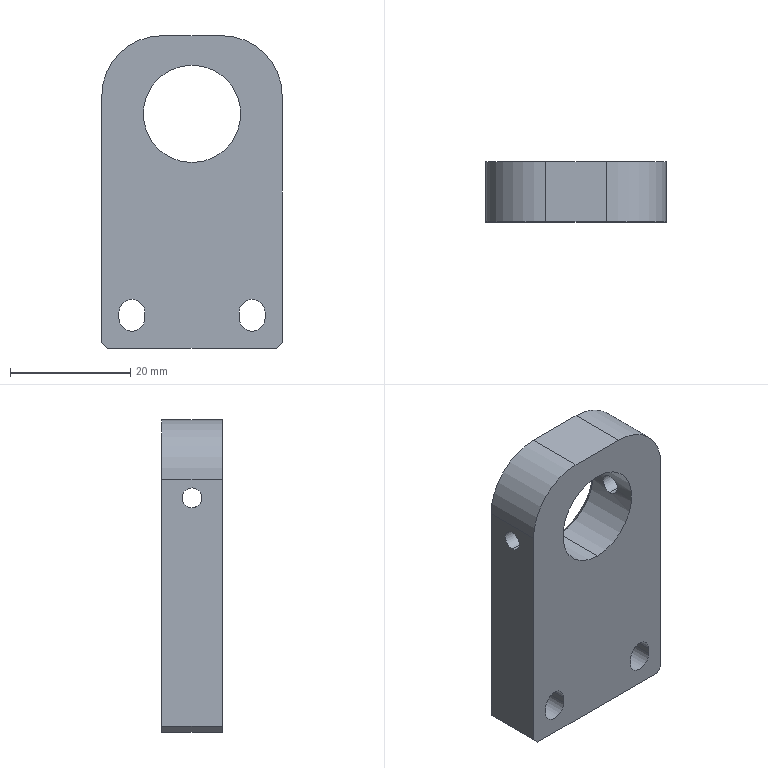Part | SolidWorks | features ICE 7, MoveFace 5, Chamfer 3, HoleWzd 3, Fillet 2, 3DProfileFeature 1, Extrusion 1, LPattern 1 | 1 solid | 40 faces | box 30 x 10 x 52 mm | volume 12313 mm3 | cylinder 20 | plane 18 | cone 2 | commonest cylinder face diameters 4.3 x6 3.3 x4 7 x3 8 x3 16.2 x2 20 x2
STEP:
#1=CARTESIAN_POINT('',(15.,11.,30.9));
#2=VERTEX_POINT('',#1);
#3=CARTESIAN_POINT('',(15.,11.,47.1));
#4=VERTEX_POINT('',#3);
#5=CARTESIAN_POINT('',(15.,11.,39.));
#6=DIRECTION('',(0.,1.,0.));
#7=DIRECTION('',(0.,0.,-1.));
#8=AXIS2_PLACEMENT_3D('',#5,#6,#7);
#9=CIRCLE('',#8,8.1);
#10=EDGE_CURVE('',#2,#4,#9,.T.);
#11=ORIENTED_EDGE('',*,*,#10,.F.);
#12=CARTESIAN_POINT('',(15.,12.,29.9));
#13=VERTEX_POINT('',#12);
#14=CARTESIAN_POINT('',(15.,11.,30.9));
#15=DIRECTION('',(0.,0.7071,-0.7071));
#16=VECTOR('',#15,1000.);
#17=LINE('',#14,#16);
#18=EDGE_CURVE('',#2,#13,#17,.T.);
#19=ORIENTED_EDGE('',*,*,#18,.T.);
#20=CARTESIAN_POINT('',(15.,12.,48.1));
#21=VERTEX_POINT('',#20);
#22=CARTESIAN_POINT('',(15.,12.,39.));
#23=DIRECTION('',(0.,-1.,0.));
#24=DIRECTION('',(0.,0.,-1.));
#25=AXIS2_PLACEMENT_3D('',#22,#23,#24);
#26=CIRCLE('',#25,9.1);
#27=EDGE_CURVE('',#21,#13,#26,.T.);
#28=ORIENTED_EDGE('',*,*,#27,.F.);
#29=CARTESIAN_POINT('',(15.,11.,47.1));
#30=DIRECTION('',(0.,0.7071,0.7071));
#31=VECTOR('',#30,1000.);
#32=LINE('',#29,#31);
#33=EDGE_CURVE('',#4,#21,#32,.T.);
#34=ORIENTED_EDGE('',*,*,#33,.F.);
#35=EDGE_LOOP('',(#11,#19,#28,#34));
#36=FACE_OUTER_BOUND('',#35,.T.);
#37=CARTESIAN_POINT('',(15.,11.,39.));
#38=DIRECTION('',(0.,1.,0.));
#39=DIRECTION('',(0.,0.,1.));
#40=AXIS2_PLACEMENT_3D('',#37,#38,#39);
#41=CONICAL_SURFACE('',#40,8.1,0.7854);
#42=ADVANCED_FACE('',(#36),#41,.F.);
#43=CARTESIAN_POINT('',(25.,8.,9.5));
#44=VERTEX_POINT('',#43);
#45=CARTESIAN_POINT('',(28.5,8.,6.));
#46=VERTEX_POINT('',#45);
#47=CARTESIAN_POINT('',(25.,8.,6.));
#48=DIRECTION('',(0.,1.,0.));
#49=DIRECTION('',(0.,0.,1.));
#50=AXIS2_PLACEMENT_3D('',#47,#48,#49);
#51=CIRCLE('',#50,3.5);
#52=EDGE_CURVE('',#44,#46,#51,.T.);
#53=ORIENTED_EDGE('',*,*,#52,.F.);
#54=CARTESIAN_POINT('',(25.,12.,9.5));
#55=VERTEX_POINT('',#54);
#56=CARTESIAN_POINT('',(25.,8.,9.5));
#57=DIRECTION('',(0.,1.,0.));
#58=VECTOR('',#57,1000.);
#59=LINE('',#56,#58);
#60=EDGE_CURVE('',#44,#55,#59,.T.);
#61=ORIENTED_EDGE('',*,*,#60,.T.);
#62=CARTESIAN_POINT('',(28.5,12.,6.));
#63=VERTEX_POINT('',#62);
#64=CARTESIAN_POINT('',(25.,12.,6.));
#65=DIRECTION('',(0.,1.,0.));
#66=DIRECTION('',(0.,0.,1.));
#67=AXIS2_PLACEMENT_3D('',#64,#65,#66);
#68=CIRCLE('',#67,3.5);
#69=EDGE_CURVE('',#55,#63,#68,.T.);
#70=ORIENTED_EDGE('',*,*,#69,.T.);
#71=CARTESIAN_POINT('',(28.5,8.,6.));
#72=DIRECTION('',(0.,1.,0.));
#73=VECTOR('',#72,1000.);
#74=LINE('',#71,#73);
#75=EDGE_CURVE('',#46,#63,#74,.T.);
#76=ORIENTED_EDGE('',*,*,#75,.F.);
#77=EDGE_LOOP('',(#53,#61,#70,#76));
#78=FACE_OUTER_BOUND('',#77,.T.);
#79=CARTESIAN_POINT('',(25.,8.,6.));
#80=DIRECTION('',(0.,1.,0.));
#81=DIRECTION('',(0.,0.,1.));
#82=AXIS2_PLACEMENT_3D('',#79,#80,#81);
#83=CYLINDRICAL_SURFACE('',#82,3.5);
#84=ADVANCED_FACE('',(#78),#83,.F.);
#85=CARTESIAN_POINT('',(5.,8.,10.));
#86=VERTEX_POINT('',#85);
#87=CARTESIAN_POINT('',(9.,8.,6.));
#88=VERTEX_POINT('',#87);
#89=CARTESIAN_POINT('',(5.,8.,6.));
#90=DIRECTION('',(0.,1.,0.));
#91=DIRECTION('',(0.,0.,1.));
#92=AXIS2_PLACEMENT_3D('',#89,#90,#91);
#93=CIRCLE('',#92,4.);
#94=EDGE_CURVE('',#86,#88,#93,.T.);
#95=ORIENTED_EDGE('',*,*,#94,.F.);
#96=CARTESIAN_POINT('',(5.,12.,10.));
#97=VERTEX_POINT('',#96);
#98=CARTESIAN_POINT('',(5.,8.,10.));
#99=DIRECTION('',(0.,1.,0.));
#100=VECTOR('',#99,1000.);
#101=LINE('',#98,#100);
#102=EDGE_CURVE('',#86,#97,#101,.T.);
#103=ORIENTED_EDGE('',*,*,#102,.T.);
#104=CARTESIAN_POINT('',(9.,12.,6.));
#105=VERTEX_POINT('',#104);
#106=CARTESIAN_POINT('',(5.,12.,6.));
#107=DIRECTION('',(0.,1.,0.));
#108=DIRECTION('',(0.,0.,1.));
#109=AXIS2_PLACEMENT_3D('',#106,#107,#108);
#110=CIRCLE('',#109,4.);
#111=EDGE_CURVE('',#97,#105,#110,.T.);
#112=ORIENTED_EDGE('',*,*,#111,.T.);
#113=CARTESIAN_POINT('',(9.,8.,6.));
#114=DIRECTION('',(0.,1.,0.));
#115=VECTOR('',#114,1000.);
#116=LINE('',#113,#115);
#117=EDGE_CURVE('',#88,#105,#116,.T.);
#118=ORIENTED_EDGE('',*,*,#117,.F.);
#119=EDGE_LOOP('',(#95,#103,#112,#118));
#120=FACE_OUTER_BOUND('',#119,.T.);
#121=CARTESIAN_POINT('',(5.,8.,6.));
#122=DIRECTION('',(0.,1.,0.));
#123=DIRECTION('',(0.,0.,1.));
#124=AXIS2_PLACEMENT_3D('',#121,#122,#123);
#125=CYLINDRICAL_SURFACE('',#124,4.);
#126=ADVANCED_FACE('',(#120),#125,.F.);
#127=CARTESIAN_POINT('',(7.07,7.,37.35));
#128=VERTEX_POINT('',#127);
#129=CARTESIAN_POINT('',(7.07,7.,40.65));
#130=VERTEX_POINT('',#129);
#131=CARTESIAN_POINT('',(7.07,7.,37.35));
#132=CARTESIAN_POINT('',(7.07,6.784,37.35));
#133=CARTESIAN_POINT('',(7.06,6.567,37.393));
#134=CARTESIAN_POINT('',(7.037,6.269,37.517));
#135=CARTESIAN_POINT('',(7.027,6.172,37.568));
#136=CARTESIAN_POINT('',(7.007,5.993,37.689));
#137=CARTESIAN_POINT('',(6.996,5.91,37.757));
#138=CARTESIAN_POINT('',(6.973,5.758,37.909));
#139=CARTESIAN_POINT('',(6.962,5.688,37.993));
#140=CARTESIAN_POINT('',(6.942,5.569,38.172));
#141=CARTESIAN_POINT('',(6.933,5.518,38.266));
#142=CARTESIAN_POINT('',(6.909,5.393,38.567));
#143=CARTESIAN_POINT('',(6.9,5.35,38.781));
#144=CARTESIAN_POINT('',(6.9,5.35,39.108));
#145=CARTESIAN_POINT('',(6.902,5.361,39.215));
#146=CARTESIAN_POINT('',(6.911,5.403,39.427));
#147=CARTESIAN_POINT('',(6.917,5.434,39.532));
#148=CARTESIAN_POINT('',(6.932,5.517,39.731));
#149=CARTESIAN_POINT('',(6.942,5.568,39.826));
#150=CARTESIAN_POINT('',(6.962,5.688,40.006));
#151=CARTESIAN_POINT('',(6.973,5.757,40.09));
#152=CARTESIAN_POINT('',(7.006,5.984,40.318));
#153=CARTESIAN_POINT('',(7.029,6.168,40.441));
#154=CARTESIAN_POINT('',(7.06,6.564,40.606));
#155=CARTESIAN_POINT('',(7.07,6.781,40.65));
#156=CARTESIAN_POINT('',(7.07,7.,40.65));
#157=B_SPLINE_CURVE_WITH_KNOTS('',3,(#131,#132,#133,#134,#135,#136,#137,#138,#139,#140,#141,#142,#143,#144,#145,#146,#147,#148,#149,#150,#151,#152,#153,#154,#155,#156),.UNSPECIFIED.,.F.,.F.,(4,2,2,2,2,2,2,2,2,2,2,2,4),(0.005172,0.005819,0.006142,0.006465,0.006788,0.007111,0.007758,0.008081,0.008404,0.008727,0.00905,0.009697,0.01034),.UNSPECIFIED.);
#158=EDGE_CURVE('',#128,#130,#157,.T.);
#159=ORIENTED_EDGE('',*,*,#158,.F.);
#160=CARTESIAN_POINT('',(0.,7.,37.35));
#161=VERTEX_POINT('',#160);
#162=CARTESIAN_POINT('',(0.,7.,37.35));
#163=DIRECTION('',(-1.,0.,0.));
#164=VECTOR('',#163,1000.);
#165=LINE('',#162,#164);
#166=EDGE_CURVE('',#128,#161,#165,.T.);
#167=ORIENTED_EDGE('',*,*,#166,.T.);
#168=CARTESIAN_POINT('',(0.,7.,40.65));
#169=VERTEX_POINT('',#168);
#170=CARTESIAN_POINT('',(0.,7.,39.));
#171=DIRECTION('',(-1.,0.,0.));
#172=DIRECTION('',(0.,0.,1.));
#173=AXIS2_PLACEMENT_3D('',#170,#171,#172);
#174=CIRCLE('',#173,1.65);
#175=EDGE_CURVE('',#161,#169,#174,.T.);
#176=ORIENTED_EDGE('',*,*,#175,.T.);
#177=CARTESIAN_POINT('',(0.,7.,40.65));
#178=DIRECTION('',(-1.,0.,0.));
#179=VECTOR('',#178,1000.);
#180=LINE('',#177,#179);
#181=EDGE_CURVE('',#130,#169,#180,.T.);
#182=ORIENTED_EDGE('',*,*,#181,.F.);
#183=EDGE_LOOP('',(#159,#167,#176,#182));
#184=FACE_OUTER_BOUND('',#183,.T.);
#185=CARTESIAN_POINT('',(0.,7.,39.));
#186=DIRECTION('',(-1.,0.,0.));
#187=DIRECTION('',(0.,0.,1.));
#188=AXIS2_PLACEMENT_3D('',#185,#186,#187);
#189=CYLINDRICAL_SURFACE('',#188,1.65);
#190=ADVANCED_FACE('',(#184),#189,.F.);
#191=CARTESIAN_POINT('',(22.93,7.,40.65));
#192=VERTEX_POINT('',#191);
#193=CARTESIAN_POINT('',(22.93,7.,37.35));
#194=VERTEX_POINT('',#193);
#195=CARTESIAN_POINT('',(22.93,7.,40.65));
#196=CARTESIAN_POINT('',(22.93,6.784,40.65));
#197=CARTESIAN_POINT('',(22.94,6.567,40.607));
#198=CARTESIAN_POINT('',(22.963,6.269,40.483));
#199=CARTESIAN_POINT('',(22.973,6.172,40.432));
#200=CARTESIAN_POINT('',(22.993,5.993,40.311));
#201=CARTESIAN_POINT('',(23.004,5.91,40.243));
#202=CARTESIAN_POINT('',(23.027,5.758,40.091));
#203=CARTESIAN_POINT('',(23.038,5.688,40.007));
#204=CARTESIAN_POINT('',(23.058,5.569,39.828));
#205=CARTESIAN_POINT('',(23.067,5.518,39.734));
#206=CARTESIAN_POINT('',(23.091,5.393,39.433));
#207=CARTESIAN_POINT('',(23.1,5.35,39.219));
#208=CARTESIAN_POINT('',(23.1,5.35,38.892));
#209=CARTESIAN_POINT('',(23.098,5.361,38.785));
#210=CARTESIAN_POINT('',(23.089,5.403,38.573));
#211=CARTESIAN_POINT('',(23.083,5.434,38.468));
#212=CARTESIAN_POINT('',(23.068,5.517,38.269));
#213=CARTESIAN_POINT('',(23.058,5.568,38.174));
#214=CARTESIAN_POINT('',(23.038,5.688,37.994));
#215=CARTESIAN_POINT('',(23.027,5.757,37.91));
#216=CARTESIAN_POINT('',(22.994,5.984,37.682));
#217=CARTESIAN_POINT('',(22.971,6.168,37.559));
#218=CARTESIAN_POINT('',(22.94,6.564,37.394));
#219=CARTESIAN_POINT('',(22.93,6.781,37.35));
#220=CARTESIAN_POINT('',(22.93,7.,37.35));
#221=B_SPLINE_CURVE_WITH_KNOTS('',3,(#195,#196,#197,#198,#199,#200,#201,#202,#203,#204,#205,#206,#207,#208,#209,#210,#211,#212,#213,#214,#215,#216,#217,#218,#219,#220),.UNSPECIFIED.,.F.,.F.,(4,2,2,2,2,2,2,2,2,2,2,2,4),(0.005172,0.005819,0.006142,0.006465,0.006788,0.007111,0.007758,0.008081,0.008404,0.008727,0.00905,0.009697,0.01034),.UNSPECIFIED.);
#222=EDGE_CURVE('',#192,#194,#221,.T.);
#223=ORIENTED_EDGE('',*,*,#222,.F.);
#224=CARTESIAN_POINT('',(30.,7.,40.65));
#225=VERTEX_POINT('',#224);
#226=CARTESIAN_POINT('',(30.,7.,40.65));
#227=DIRECTION('',(1.,0.,0.));
#228=VECTOR('',#227,1000.);
#229=LINE('',#226,#228);
#230=EDGE_CURVE('',#192,#225,#229,.T.);
#231=ORIENTED_EDGE('',*,*,#230,.T.);
#232=CARTESIAN_POINT('',(30.,7.,37.35));
#233=VERTEX_POINT('',#232);
#234=CARTESIAN_POINT('',(30.,7.,39.));
#235=DIRECTION('',(1.,0.,0.));
#236=DIRECTION('',(0.,0.,-1.));
#237=AXIS2_PLACEMENT_3D('',#234,#235,#236);
#238=CIRCLE('',#237,1.65);
#239=EDGE_CURVE('',#225,#233,#238,.T.);
#240=ORIENTED_EDGE('',*,*,#239,.T.);
#241=CARTESIAN_POINT('',(30.,7.,37.35));
#242=DIRECTION('',(1.,0.,0.));
#243=VECTOR('',#242,1000.);
#244=LINE('',#241,#243);
#245=EDGE_CURVE('',#194,#233,#244,.T.);
#246=ORIENTED_EDGE('',*,*,#245,.F.);
#247=EDGE_LOOP('',(#223,#231,#240,#246));
#248=FACE_OUTER_BOUND('',#247,.T.);
#249=CARTESIAN_POINT('',(30.,7.,39.));
#250=DIRECTION('',(1.,0.,0.));
#251=DIRECTION('',(0.,0.,-1.));
#252=AXIS2_PLACEMENT_3D('',#249,#250,#251);
#253=CYLINDRICAL_SURFACE('',#252,1.65);
#254=ADVANCED_FACE('',(#248),#253,.F.);
#255=CARTESIAN_POINT('',(7.07,7.,40.65));
#256=CARTESIAN_POINT('',(7.07,7.109,40.65));
#257=CARTESIAN_POINT('',(7.068,7.217,40.639));
#258=CARTESIAN_POINT('',(7.059,7.428,40.597));
#259=CARTESIAN_POINT('',(7.053,7.533,40.565));
#260=CARTESIAN_POINT('',(7.037,7.733,40.482));
#261=CARTESIAN_POINT('',(7.027,7.827,40.432));
#262=CARTESIAN_POINT('',(7.007,8.007,40.312));
#263=CARTESIAN_POINT('',(6.995,8.091,40.242));
#264=CARTESIAN_POINT('',(6.962,8.319,40.015));
#265=CARTESIAN_POINT('',(6.94,8.442,39.831));
#266=CARTESIAN_POINT('',(6.909,8.606,39.434));
#267=CARTESIAN_POINT('',(6.9,8.65,39.217));
#268=CARTESIAN_POINT('',(6.9,8.65,38.893));
#269=CARTESIAN_POINT('',(6.902,8.639,38.783));
#270=CARTESIAN_POINT('',(6.911,8.597,38.571));
#271=CARTESIAN_POINT('',(6.917,8.566,38.468));
#272=CARTESIAN_POINT('',(6.94,8.441,38.168));
#273=CARTESIAN_POINT('',(6.962,8.32,37.986));
#274=CARTESIAN_POINT('',(6.996,8.09,37.756));
#275=CARTESIAN_POINT('',(7.007,8.007,37.688));
#276=CARTESIAN_POINT('',(7.027,7.828,37.569));
#277=CARTESIAN_POINT('',(7.037,7.732,37.517));
#278=CARTESIAN_POINT('',(7.053,7.532,37.435));
#279=CARTESIAN_POINT('',(7.059,7.429,37.403));
#280=CARTESIAN_POINT('',(7.068,7.217,37.361));
#281=CARTESIAN_POINT('',(7.07,7.108,37.35));
#282=CARTESIAN_POINT('',(7.07,7.,37.35));
#283=B_SPLINE_CURVE_WITH_KNOTS('',3,(#255,#256,#257,#258,#259,#260,#261,#262,#263,#264,#265,#266,#267,#268,#269,#270,#271,#272,#273,#274,#275,#276,#277,#278,#279,#280,#281,#282),.UNSPECIFIED.,.F.,.F.,(4,2,2,2,2,2,2,2,2,2,2,2,2,4),(0.,0.0003233,0.0006465,0.0009698,0.001293,0.00194,0.002586,0.002909,0.003233,0.003879,0.004202,0.004526,0.004849,0.005172),.UNSPECIFIED.);
#284=EDGE_CURVE('',#130,#128,#283,.T.);
#285=ORIENTED_EDGE('',*,*,#284,.T.);
#286=ORIENTED_EDGE('',*,*,#158,.T.);
#287=EDGE_LOOP('',(#285,#286));
#288=FACE_BOUND('',#287,.T.);
#289=CARTESIAN_POINT('',(15.,2.,47.1));
#290=VERTEX_POINT('',#289);
#291=CARTESIAN_POINT('',(15.,2.,30.9));
#292=VERTEX_POINT('',#291);
#293=CARTESIAN_POINT('',(15.,2.,39.));
#294=DIRECTION('',(0.,-1.,0.));
#295=DIRECTION('',(0.,0.,1.));
#296=AXIS2_PLACEMENT_3D('',#293,#294,#295);
#297=CIRCLE('',#296,8.1);
#298=EDGE_CURVE('',#290,#292,#297,.T.);
#299=ORIENTED_EDGE('',*,*,#298,.T.);
#300=CARTESIAN_POINT('',(15.,-5.,30.9));
#301=DIRECTION('',(0.,1.,0.));
#302=VECTOR('',#301,1000.);
#303=LINE('',#300,#302);
#304=EDGE_CURVE('',#292,#2,#303,.T.);
#305=ORIENTED_EDGE('',*,*,#304,.T.);
#306=ORIENTED_EDGE('',*,*,#10,.T.);
#307=CARTESIAN_POINT('',(15.,-5.,47.1));
#308=DIRECTION('',(0.,1.,0.));
#309=VECTOR('',#308,1000.);
#310=LINE('',#307,#309);
#311=EDGE_CURVE('',#290,#4,#310,.T.);
#312=ORIENTED_EDGE('',*,*,#311,.F.);
#313=EDGE_LOOP('',(#299,#305,#306,#312));
#314=FACE_OUTER_BOUND('',#313,.T.);
#315=CARTESIAN_POINT('',(15.,-5.,39.));
#316=DIRECTION('',(0.,1.,0.));
#317=DIRECTION('',(0.,0.,1.));
#318=AXIS2_PLACEMENT_3D('',#315,#316,#317);
#319=CYLINDRICAL_SURFACE('',#318,8.1);
#320=ADVANCED_FACE('',(#288,#314),#319,.F.);
#321=CARTESIAN_POINT('',(5.,2.,8.15));
#322=VERTEX_POINT('',#321);
#323=CARTESIAN_POINT('',(7.15,2.,6.));
#324=VERTEX_POINT('',#323);
#325=CARTESIAN_POINT('',(5.,2.,6.));
#326=DIRECTION('',(0.,1.,0.));
#327=DIRECTION('',(0.,0.,1.));
#328=AXIS2_PLACEMENT_3D('',#325,#326,#327);
#329=CIRCLE('',#328,2.15);
#330=EDGE_CURVE('',#322,#324,#329,.T.);
#331=ORIENTED_EDGE('',*,*,#330,.F.);
#332=CARTESIAN_POINT('',(5.,8.,8.15));
#333=VERTEX_POINT('',#332);
#334=CARTESIAN_POINT('',(5.,-61.,8.15));
#335=DIRECTION('',(0.,1.,0.));
#336=VECTOR('',#335,1000.);
#337=LINE('',#334,#336);
#338=EDGE_CURVE('',#322,#333,#337,.T.);
#339=ORIENTED_EDGE('',*,*,#338,.T.);
#340=CARTESIAN_POINT('',(7.15,8.,6.));
#341=VERTEX_POINT('',#340);
#342=CARTESIAN_POINT('',(5.,8.,6.));
#343=DIRECTION('',(0.,-1.,0.));
#344=DIRECTION('',(0.,0.,1.));
#345=AXIS2_PLACEMENT_3D('',#342,#343,#344);
#346=CIRCLE('',#345,2.15);
#347=EDGE_CURVE('',#341,#333,#346,.T.);
#348=ORIENTED_EDGE('',*,*,#347,.F.);
#349=CARTESIAN_POINT('',(7.15,-61.,6.));
#350=DIRECTION('',(0.,1.,0.));
#351=VECTOR('',#350,1000.);
#352=LINE('',#349,#351);
#353=EDGE_CURVE('',#324,#341,#352,.T.);
#354=ORIENTED_EDGE('',*,*,#353,.F.);
#355=EDGE_LOOP('',(#331,#339,#348,#354));
#356=FACE_OUTER_BOUND('',#355,.T.);
#357=CARTESIAN_POINT('',(5.,-61.,6.));
#358=DIRECTION('',(0.,1.,0.));
#359=DIRECTION('',(0.,0.,1.));
#360=AXIS2_PLACEMENT_3D('',#357,#358,#359);
#361=CYLINDRICAL_SURFACE('',#360,2.15);
#362=ADVANCED_FACE('',(#356),#361,.F.);
#363=CARTESIAN_POINT('',(25.,2.,8.15));
#364=VERTEX_POINT('',#363);
#365=CARTESIAN_POINT('',(27.15,2.,6.));
#366=VERTEX_POINT('',#365);
#367=CARTESIAN_POINT('',(25.,2.,6.));
#368=DIRECTION('',(0.,1.,0.));
#369=DIRECTION('',(0.,0.,1.));
#370=AXIS2_PLACEMENT_3D('',#367,#368,#369);
#371=CIRCLE('',#370,2.15);
#372=EDGE_CURVE('',#364,#366,#371,.T.);
#373=ORIENTED_EDGE('',*,*,#372,.F.);
#374=CARTESIAN_POINT('',(25.,8.,8.15));
#375=VERTEX_POINT('',#374);
#376=CARTESIAN_POINT('',(25.,-61.,8.15));
#377=DIRECTION('',(0.,1.,0.));
#378=VECTOR('',#377,1000.);
#379=LINE('',#376,#378);
#380=EDGE_CURVE('',#364,#375,#379,.T.);
#381=ORIENTED_EDGE('',*,*,#380,.T.);
#382=CARTESIAN_POINT('',(27.15,8.,6.));
#383=VERTEX_POINT('',#382);
#384=CARTESIAN_POINT('',(25.,8.,6.));
#385=DIRECTION('',(0.,-1.,0.));
#386=DIRECTION('',(0.,0.,1.));
#387=AXIS2_PLACEMENT_3D('',#384,#385,#386);
#388=CIRCLE('',#387,2.15);
#389=EDGE_CURVE('',#383,#375,#388,.T.);
#390=ORIENTED_EDGE('',*,*,#389,.F.);
#391=CARTESIAN_POINT('',(27.15,-61.,6.));
#392=DIRECTION('',(0.,1.,0.));
#393=VECTOR('',#392,1000.);
#394=LINE('',#391,#393);
#395=EDGE_CURVE('',#366,#383,#394,.T.);
#396=ORIENTED_EDGE('',*,*,#395,.F.);
#397=EDGE_LOOP('',(#373,#381,#390,#396));
#398=FACE_OUTER_BOUND('',#397,.T.);
#399=CARTESIAN_POINT('',(25.,-61.,6.));
#400=DIRECTION('',(0.,1.,0.));
#401=DIRECTION('',(0.,0.,1.));
#402=AXIS2_PLACEMENT_3D('',#399,#400,#401);
#403=CYLINDRICAL_SURFACE('',#402,2.15);
#404=ADVANCED_FACE('',(#398),#403,.F.);
#405=CARTESIAN_POINT('',(22.85,8.,5.));
#406=VERTEX_POINT('',#405);
#407=CARTESIAN_POINT('',(27.15,8.,5.));
#408=VERTEX_POINT('',#407);
#409=CARTESIAN_POINT('',(25.,8.,5.));
#410=DIRECTION('',(0.,-1.,0.));
#411=DIRECTION('',(0.,0.,1.));
#412=AXIS2_PLACEMENT_3D('',#409,#410,#411);
#413=CIRCLE('',#412,2.15);
#414=EDGE_CURVE('',#406,#408,#413,.T.);
#415=ORIENTED_EDGE('',*,*,#414,.F.);
#416=CARTESIAN_POINT('',(22.85,2.,5.));
#417=VERTEX_POINT('',#416);
#418=CARTESIAN_POINT('',(22.85,-61.,5.));
#419=DIRECTION('',(0.,1.,0.));
#420=VECTOR('',#419,1000.);
#421=LINE('',#418,#420);
#422=EDGE_CURVE('',#417,#406,#421,.T.);
#423=ORIENTED_EDGE('',*,*,#422,.F.);
#424=CARTESIAN_POINT('',(27.15,2.,5.));
#425=VERTEX_POINT('',#424);
#426=CARTESIAN_POINT('',(25.,2.,5.));
#427=DIRECTION('',(0.,1.,0.));
#428=DIRECTION('',(0.,0.,1.));
#429=AXIS2_PLACEMENT_3D('',#426,#427,#428);
#430=CIRCLE('',#429,2.15);
#431=EDGE_CURVE('',#425,#417,#430,.T.);
#432=ORIENTED_EDGE('',*,*,#431,.F.);
#433=CARTESIAN_POINT('',(27.15,-61.,5.));
#434=DIRECTION('',(0.,1.,0.));
#435=VECTOR('',#434,1000.);
#436=LINE('',#433,#435);
#437=EDGE_CURVE('',#425,#408,#436,.T.);
#438=ORIENTED_EDGE('',*,*,#437,.T.);
#439=EDGE_LOOP('',(#415,#423,#432,#438));
#440=FACE_OUTER_BOUND('',#439,.T.);
#441=CARTESIAN_POINT('',(25.,-61.,5.));
#442=DIRECTION('',(0.,1.,0.));
#443=DIRECTION('',(0.,0.,1.));
#444=AXIS2_PLACEMENT_3D('',#441,#442,#443);
#445=CYLINDRICAL_SURFACE('',#444,2.15);
#446=ADVANCED_FACE('',(#440),#445,.F.);
#447=CARTESIAN_POINT('',(27.15,8.,4.));
#448=DIRECTION('',(0.,0.,1.));
#449=VECTOR('',#448,1000.);
#450=LINE('',#447,#449);
#451=EDGE_CURVE('',#408,#383,#450,.T.);
#452=ORIENTED_EDGE('',*,*,#451,.F.);
#453=ORIENTED_EDGE('',*,*,#437,.F.);
#454=CARTESIAN_POINT('',(27.15,2.,56.52));
#455=DIRECTION('',(0.,0.,-1.));
#456=VECTOR('',#455,1000.);
#457=LINE('',#454,#456);
#458=EDGE_CURVE('',#366,#425,#457,.T.);
#459=ORIENTED_EDGE('',*,*,#458,.F.);
#460=ORIENTED_EDGE('',*,*,#395,.T.);
#461=EDGE_LOOP('',(#452,#453,#459,#460));
#462=FACE_OUTER_BOUND('',#461,.T.);
#463=CARTESIAN_POINT('',(27.15,-61.,4.));
#464=DIRECTION('',(1.,0.,0.));
#465=DIRECTION('',(0.,0.,-1.));
#466=AXIS2_PLACEMENT_3D('',#463,#464,#465);
#467=PLANE('',#466);
#468=ADVANCED_FACE('',(#462),#467,.F.);
#469=ORIENTED_EDGE('',*,*,#380,.F.);
#470=CARTESIAN_POINT('',(22.85,2.,6.));
#471=VERTEX_POINT('',#470);
#472=CARTESIAN_POINT('',(25.,2.,6.));
#473=DIRECTION('',(0.,1.,0.));
#474=DIRECTION('',(0.,0.,1.));
#475=AXIS2_PLACEMENT_3D('',#472,#473,#474);
#476=CIRCLE('',#475,2.15);
#477=EDGE_CURVE('',#471,#364,#476,.T.);
#478=ORIENTED_EDGE('',*,*,#477,.F.);
#479=CARTESIAN_POINT('',(22.85,8.,6.));
#480=VERTEX_POINT('',#479);
#481=CARTESIAN_POINT('',(22.85,-61.,6.));
#482=DIRECTION('',(0.,1.,0.));
#483=VECTOR('',#482,1000.);
#484=LINE('',#481,#483);
#485=EDGE_CURVE('',#471,#480,#484,.T.);
#486=ORIENTED_EDGE('',*,*,#485,.T.);
#487=CARTESIAN_POINT('',(25.,8.,6.));
#488=DIRECTION('',(0.,-1.,0.));
#489=DIRECTION('',(0.,0.,1.));
#490=AXIS2_PLACEMENT_3D('',#487,#488,#489);
#491=CIRCLE('',#490,2.15);
#492=EDGE_CURVE('',#375,#480,#491,.T.);
#493=ORIENTED_EDGE('',*,*,#492,.F.);
#494=EDGE_LOOP('',(#469,#478,#486,#493));
#495=FACE_OUTER_BOUND('',#494,.T.);
#496=CARTESIAN_POINT('',(25.,-61.,6.));
#497=DIRECTION('',(0.,1.,0.));
#498=DIRECTION('',(0.,0.,1.));
#499=AXIS2_PLACEMENT_3D('',#496,#497,#498);
#500=CYLINDRICAL_SURFACE('',#499,2.15);
#501=ADVANCED_FACE('',(#495),#500,.F.);
#502=CARTESIAN_POINT('',(22.85,8.,4.));
#503=DIRECTION('',(0.,0.,-1.));
#504=VECTOR('',#503,1000.);
#505=LINE('',#502,#504);
#506=EDGE_CURVE('',#480,#406,#505,.T.);
#507=ORIENTED_EDGE('',*,*,#506,.F.);
#508=ORIENTED_EDGE('',*,*,#485,.F.);
#509=CARTESIAN_POINT('',(22.85,2.,56.52));
#510=DIRECTION('',(0.,0.,1.));
#511=VECTOR('',#510,1000.);
#512=LINE('',#509,#511);
#513=EDGE_CURVE('',#417,#471,#512,.T.);
#514=ORIENTED_EDGE('',*,*,#513,.F.);
#515=ORIENTED_EDGE('',*,*,#422,.T.);
#516=EDGE_LOOP('',(#507,#508,#514,#515));
#517=FACE_OUTER_BOUND('',#516,.T.);
#518=CARTESIAN_POINT('',(22.85,-61.,4.));
#519=DIRECTION('',(-1.,0.,0.));
#520=DIRECTION('',(0.,0.,1.));
#521=AXIS2_PLACEMENT_3D('',#518,#519,#520);
#522=PLANE('',#521);
#523=ADVANCED_FACE('',(#517),#522,.F.);
#524=CARTESIAN_POINT('',(2.85,8.,5.));
#525=VERTEX_POINT('',#524);
#526=CARTESIAN_POINT('',(7.15,8.,5.));
#527=VERTEX_POINT('',#526);
#528=CARTESIAN_POINT('',(5.,8.,5.));
#529=DIRECTION('',(0.,-1.,0.));
#530=DIRECTION('',(0.,0.,1.));
#531=AXIS2_PLACEMENT_3D('',#528,#529,#530);
#532=CIRCLE('',#531,2.15);
#533=EDGE_CURVE('',#525,#527,#532,.T.);
#534=ORIENTED_EDGE('',*,*,#533,.F.);
#535=CARTESIAN_POINT('',(2.85,2.,5.));
#536=VERTEX_POINT('',#535);
#537=CARTESIAN_POINT('',(2.85,-61.,5.));
#538=DIRECTION('',(0.,1.,0.));
#539=VECTOR('',#538,1000.);
#540=LINE('',#537,#539);
#541=EDGE_CURVE('',#536,#525,#540,.T.);
#542=ORIENTED_EDGE('',*,*,#541,.F.);
#543=CARTESIAN_POINT('',(7.15,2.,5.));
#544=VERTEX_POINT('',#543);
#545=CARTESIAN_POINT('',(5.,2.,5.));
#546=DIRECTION('',(0.,1.,0.));
#547=DIRECTION('',(0.,0.,1.));
#548=AXIS2_PLACEMENT_3D('',#545,#546,#547);
#549=CIRCLE('',#548,2.15);
#550=EDGE_CURVE('',#544,#536,#549,.T.);
#551=ORIENTED_EDGE('',*,*,#550,.F.);
#552=CARTESIAN_POINT('',(7.15,-61.,5.));
#553=DIRECTION('',(0.,1.,0.));
#554=VECTOR('',#553,1000.);
#555=LINE('',#552,#554);
#556=EDGE_CURVE('',#544,#527,#555,.T.);
#557=ORIENTED_EDGE('',*,*,#556,.T.);
#558=EDGE_LOOP('',(#534,#542,#551,#557));
#559=FACE_OUTER_BOUND('',#558,.T.);
#560=CARTESIAN_POINT('',(5.,-61.,5.));
#561=DIRECTION('',(0.,1.,0.));
#562=DIRECTION('',(0.,0.,1.));
#563=AXIS2_PLACEMENT_3D('',#560,#561,#562);
#564=CYLINDRICAL_SURFACE('',#563,2.15);
#565=ADVANCED_FACE('',(#559),#564,.F.);
#566=CARTESIAN_POINT('',(7.15,8.,4.));
#567=DIRECTION('',(0.,0.,1.));
#568=VECTOR('',#567,1000.);
#569=LINE('',#566,#568);
#570=EDGE_CURVE('',#527,#341,#569,.T.);
#571=ORIENTED_EDGE('',*,*,#570,.F.);
#572=ORIENTED_EDGE('',*,*,#556,.F.);
#573=CARTESIAN_POINT('',(7.15,2.,56.52));
#574=DIRECTION('',(0.,0.,-1.));
#575=VECTOR('',#574,1000.);
#576=LINE('',#573,#575);
#577=EDGE_CURVE('',#324,#544,#576,.T.);
#578=ORIENTED_EDGE('',*,*,#577,.F.);
#579=ORIENTED_EDGE('',*,*,#353,.T.);
#580=EDGE_LOOP('',(#571,#572,#578,#579));
#581=FACE_OUTER_BOUND('',#580,.T.);
#582=CARTESIAN_POINT('',(7.15,-61.,4.));
#583=DIRECTION('',(1.,0.,0.));
#584=DIRECTION('',(0.,0.,-1.));
#585=AXIS2_PLACEMENT_3D('',#582,#583,#584);
#586=PLANE('',#585);
#587=ADVANCED_FACE('',(#581),#586,.F.);
#588=ORIENTED_EDGE('',*,*,#338,.F.);
#589=CARTESIAN_POINT('',(2.85,2.,6.));
#590=VERTEX_POINT('',#589);
#591=CARTESIAN_POINT('',(5.,2.,6.));
#592=DIRECTION('',(0.,1.,0.));
#593=DIRECTION('',(0.,0.,1.));
#594=AXIS2_PLACEMENT_3D('',#591,#592,#593);
#595=CIRCLE('',#594,2.15);
#596=EDGE_CURVE('',#590,#322,#595,.T.);
#597=ORIENTED_EDGE('',*,*,#596,.F.);
#598=CARTESIAN_POINT('',(2.85,8.,6.));
#599=VERTEX_POINT('',#598);
#600=CARTESIAN_POINT('',(2.85,-61.,6.));
#601=DIRECTION('',(0.,1.,0.));
#602=VECTOR('',#601,1000.);
#603=LINE('',#600,#602);
#604=EDGE_CURVE('',#590,#599,#603,.T.);
#605=ORIENTED_EDGE('',*,*,#604,.T.);
#606=CARTESIAN_POINT('',(5.,8.,6.));
#607=DIRECTION('',(0.,-1.,0.));
#608=DIRECTION('',(0.,0.,1.));
#609=AXIS2_PLACEMENT_3D('',#606,#607,#608);
#610=CIRCLE('',#609,2.15);
#611=EDGE_CURVE('',#333,#599,#610,.T.);
#612=ORIENTED_EDGE('',*,*,#611,.F.);
#613=EDGE_LOOP('',(#588,#597,#605,#612));
#614=FACE_OUTER_BOUND('',#613,.T.);
#615=CARTESIAN_POINT('',(5.,-61.,6.));
#616=DIRECTION('',(0.,1.,0.));
#617=DIRECTION('',(0.,0.,1.));
#618=AXIS2_PLACEMENT_3D('',#615,#616,#617);
#619=CYLINDRICAL_SURFACE('',#618,2.15);
#620=ADVANCED_FACE('',(#614),#619,.F.);
#621=CARTESIAN_POINT('',(2.85,8.,4.));
#622=DIRECTION('',(0.,0.,-1.));
#623=VECTOR('',#622,1000.);
#624=LINE('',#621,#623);
#625=EDGE_CURVE('',#599,#525,#624,.T.);
#626=ORIENTED_EDGE('',*,*,#625,.F.);
#627=ORIENTED_EDGE('',*,*,#604,.F.);
#628=CARTESIAN_POINT('',(2.85,2.,56.52));
#629=DIRECTION('',(0.,0.,1.));
#630=VECTOR('',#629,1000.);
#631=LINE('',#628,#630);
#632=EDGE_CURVE('',#536,#590,#631,.T.);
#633=ORIENTED_EDGE('',*,*,#632,.F.);
#634=ORIENTED_EDGE('',*,*,#541,.T.);
#635=EDGE_LOOP('',(#626,#627,#633,#634));
#636=FACE_OUTER_BOUND('',#635,.T.);
#637=CARTESIAN_POINT('',(2.85,-61.,4.));
#638=DIRECTION('',(-1.,0.,0.));
#639=DIRECTION('',(0.,0.,1.));
#640=AXIS2_PLACEMENT_3D('',#637,#638,#639);
#641=PLANE('',#640);
#642=ADVANCED_FACE('',(#636),#641,.F.);
#643=CARTESIAN_POINT('',(0.,2.,1.));
#644=VERTEX_POINT('',#643);
#645=CARTESIAN_POINT('',(0.,2.,42.));
#646=VERTEX_POINT('',#645);
#647=CARTESIAN_POINT('',(0.,2.,52.));
#648=DIRECTION('',(0.,0.,1.));
#649=VECTOR('',#648,1000.);
#650=LINE('',#647,#649);
#651=EDGE_CURVE('',#644,#646,#650,.T.);
#652=ORIENTED_EDGE('',*,*,#651,.T.);
#653=CARTESIAN_POINT('',(0.,12.,42.));
#654=VERTEX_POINT('',#653);
#655=CARTESIAN_POINT('',(0.,12.,42.));
#656=DIRECTION('',(0.,1.,0.));
#657=VECTOR('',#656,1000.);
#658=LINE('',#655,#657);
#659=EDGE_CURVE('',#646,#654,#658,.T.);
#660=ORIENTED_EDGE('',*,*,#659,.T.);
#661=CARTESIAN_POINT('',(0.,12.,1.));
#662=VERTEX_POINT('',#661);
#663=CARTESIAN_POINT('',(0.,12.,52.));
#664=DIRECTION('',(0.,0.,1.));
#665=VECTOR('',#664,1000.);
#666=LINE('',#663,#665);
#667=EDGE_CURVE('',#662,#654,#666,.T.);
#668=ORIENTED_EDGE('',*,*,#667,.F.);
#669=CARTESIAN_POINT('',(0.,12.,1.));
#670=DIRECTION('',(0.,-1.,0.));
#671=VECTOR('',#670,1000.);
#672=LINE('',#669,#671);
#673=EDGE_CURVE('',#662,#644,#672,.T.);
#674=ORIENTED_EDGE('',*,*,#673,.T.);
#675=EDGE_LOOP('',(#652,#660,#668,#674));
#676=FACE_OUTER_BOUND('',#675,.T.);
#677=CARTESIAN_POINT('',(0.,7.,39.));
#678=DIRECTION('',(-1.,0.,0.));
#679=DIRECTION('',(0.,0.,1.));
#680=AXIS2_PLACEMENT_3D('',#677,#678,#679);
#681=CIRCLE('',#680,1.65);
#682=EDGE_CURVE('',#169,#161,#681,.T.);
#683=ORIENTED_EDGE('',*,*,#682,.F.);
#684=ORIENTED_EDGE('',*,*,#175,.F.);
#685=EDGE_LOOP('',(#683,#684));
#686=FACE_BOUND('',#685,.T.);
#687=CARTESIAN_POINT('',(0.,12.,52.));
#688=DIRECTION('',(1.,0.,0.));
#689=DIRECTION('',(0.,0.,-1.));
#690=AXIS2_PLACEMENT_3D('',#687,#688,#689);
#691=PLANE('',#690);
#692=ADVANCED_FACE('',(#676,#686),#691,.F.);
#693=CARTESIAN_POINT('',(29.,12.,0.));
#694=VERTEX_POINT('',#693);
#695=CARTESIAN_POINT('',(29.,2.,0.));
#696=VERTEX_POINT('',#695);
#697=CARTESIAN_POINT('',(29.,12.,0.));
#698=DIRECTION('',(0.,-1.,0.));
#699=VECTOR('',#698,1000.);
#700=LINE('',#697,#699);
#701=EDGE_CURVE('',#694,#696,#700,.T.);
#702=ORIENTED_EDGE('',*,*,#701,.T.);
#703=CARTESIAN_POINT('',(1.,2.,0.));
#704=VERTEX_POINT('',#703);
#705=CARTESIAN_POINT('',(0.,2.,0.));
#706=DIRECTION('',(-1.,0.,0.));
#707=VECTOR('',#706,1000.);
#708=LINE('',#705,#707);
#709=EDGE_CURVE('',#696,#704,#708,.T.);
#710=ORIENTED_EDGE('',*,*,#709,.T.);
#711=CARTESIAN_POINT('',(1.,12.,0.));
#712=VERTEX_POINT('',#711);
#713=CARTESIAN_POINT('',(1.,12.,0.));
#714=DIRECTION('',(0.,1.,0.));
#715=VECTOR('',#714,1000.);
#716=LINE('',#713,#715);
#717=EDGE_CURVE('',#704,#712,#716,.T.);
#718=ORIENTED_EDGE('',*,*,#717,.T.);
#719=CARTESIAN_POINT('',(0.,12.,0.));
#720=DIRECTION('',(-1.,0.,0.));
#721=VECTOR('',#720,1000.);
#722=LINE('',#719,#721);
#723=EDGE_CURVE('',#694,#712,#722,.T.);
#724=ORIENTED_EDGE('',*,*,#723,.F.);
#725=EDGE_LOOP('',(#702,#710,#718,#724));
#726=FACE_OUTER_BOUND('',#725,.T.);
#727=CARTESIAN_POINT('',(0.,12.,0.));
#728=DIRECTION('',(0.,0.,1.));
#729=DIRECTION('',(1.,0.,0.));
#730=AXIS2_PLACEMENT_3D('',#727,#728,#729);
#731=PLANE('',#730);
#732=ADVANCED_FACE('',(#726),#731,.F.);
#733=CARTESIAN_POINT('',(10.,12.,52.));
#734=VERTEX_POINT('',#733);
#735=CARTESIAN_POINT('',(20.,12.,52.));
#736=VERTEX_POINT('',#735);
#737=CARTESIAN_POINT('',(30.,12.,52.));
#738=DIRECTION('',(1.,0.,0.));
#739=VECTOR('',#738,1000.);
#740=LINE('',#737,#739);
#741=EDGE_CURVE('',#734,#736,#740,.T.);
#742=ORIENTED_EDGE('',*,*,#741,.F.);
#743=CARTESIAN_POINT('',(10.,2.,52.));
#744=VERTEX_POINT('',#743);
#745=CARTESIAN_POINT('',(10.,12.,52.));
#746=DIRECTION('',(0.,-1.,0.));
#747=VECTOR('',#746,1000.);
#748=LINE('',#745,#747);
#749=EDGE_CURVE('',#734,#744,#748,.T.);
#750=ORIENTED_EDGE('',*,*,#749,.T.);
#751=CARTESIAN_POINT('',(20.,2.,52.));
#752=VERTEX_POINT('',#751);
#753=CARTESIAN_POINT('',(30.,2.,52.));
#754=DIRECTION('',(1.,0.,0.));
#755=VECTOR('',#754,1000.);
#756=LINE('',#753,#755);
#757=EDGE_CURVE('',#744,#752,#756,.T.);
#758=ORIENTED_EDGE('',*,*,#757,.T.);
#759=CARTESIAN_POINT('',(20.,12.,52.));
#760=DIRECTION('',(0.,1.,0.));
#761=VECTOR('',#760,1000.);
#762=LINE('',#759,#761);
#763=EDGE_CURVE('',#752,#736,#762,.T.);
#764=ORIENTED_EDGE('',*,*,#763,.T.);
#765=EDGE_LOOP('',(#742,#750,#758,#764));
#766=FACE_OUTER_BOUND('',#765,.T.);
#767=CARTESIAN_POINT('',(30.,12.,52.));
#768=DIRECTION('',(0.,0.,-1.));
#769=DIRECTION('',(-1.,0.,0.));
#770=AXIS2_PLACEMENT_3D('',#767,#768,#769);
#771=PLANE('',#770);
#772=ADVANCED_FACE('',(#766),#771,.F.);
#773=CARTESIAN_POINT('',(30.,7.,39.));
#774=DIRECTION('',(1.,0.,0.));
#775=DIRECTION('',(0.,0.,-1.));
#776=AXIS2_PLACEMENT_3D('',#773,#774,#775);
#777=CIRCLE('',#776,1.65);
#778=EDGE_CURVE('',#233,#225,#777,.T.);
#779=ORIENTED_EDGE('',*,*,#778,.F.);
#780=ORIENTED_EDGE('',*,*,#239,.F.);
#781=EDGE_LOOP('',(#779,#780));
#782=FACE_BOUND('',#781,.T.);
#783=CARTESIAN_POINT('',(30.,12.,42.));
#784=VERTEX_POINT('',#783);
#785=CARTESIAN_POINT('',(30.,12.,1.));
#786=VERTEX_POINT('',#785);
#787=CARTESIAN_POINT('',(30.,12.,10.));
#788=DIRECTION('',(0.,0.,-1.));
#789=VECTOR('',#788,1000.);
#790=LINE('',#787,#789);
#791=EDGE_CURVE('',#784,#786,#790,.T.);
#792=ORIENTED_EDGE('',*,*,#791,.F.);
#793=CARTESIAN_POINT('',(30.,2.,42.));
#794=VERTEX_POINT('',#793);
#795=CARTESIAN_POINT('',(30.,12.,42.));
#796=DIRECTION('',(0.,-1.,0.));
#797=VECTOR('',#796,1000.);
#798=LINE('',#795,#797);
#799=EDGE_CURVE('',#784,#794,#798,.T.);
#800=ORIENTED_EDGE('',*,*,#799,.T.);
#801=CARTESIAN_POINT('',(30.,2.,1.));
#802=VERTEX_POINT('',#801);
#803=CARTESIAN_POINT('',(30.,2.,56.52));
#804=DIRECTION('',(0.,0.,1.));
#805=VECTOR('',#804,1000.);
#806=LINE('',#803,#805);
#807=EDGE_CURVE('',#802,#794,#806,.T.);
#808=ORIENTED_EDGE('',*,*,#807,.F.);
#809=CARTESIAN_POINT('',(30.,12.,1.));
#810=DIRECTION('',(0.,1.,0.));
#811=VECTOR('',#810,1000.);
#812=LINE('',#809,#811);
#813=EDGE_CURVE('',#802,#786,#812,.T.);
#814=ORIENTED_EDGE('',*,*,#813,.T.);
#815=EDGE_LOOP('',(#792,#800,#808,#814));
#816=FACE_OUTER_BOUND('',#815,.T.);
#817=CARTESIAN_POINT('',(30.,12.,10.));
#818=DIRECTION('',(-1.,0.,0.));
#819=DIRECTION('',(0.,0.,1.));
#820=AXIS2_PLACEMENT_3D('',#817,#818,#819);
#821=PLANE('',#820);
#822=ADVANCED_FACE('',(#782,#816),#821,.F.);
#823=ORIENTED_EDGE('',*,*,#27,.T.);
#824=CARTESIAN_POINT('',(15.,12.,39.));
#825=DIRECTION('',(0.,-1.,0.));
#826=DIRECTION('',(0.,0.,-1.));
#827=AXIS2_PLACEMENT_3D('',#824,#825,#826);
#828=CIRCLE('',#827,9.1);
#829=EDGE_CURVE('',#13,#21,#828,.T.);
#830=ORIENTED_EDGE('',*,*,#829,.T.);
#831=EDGE_LOOP('',(#823,#830));
#832=FACE_BOUND('',#831,.T.);
#833=CARTESIAN_POINT('',(21.5,12.,5.));
#834=VERTEX_POINT('',#833);
#835=CARTESIAN_POINT('',(21.5,12.,6.));
#836=VERTEX_POINT('',#835);
#837=CARTESIAN_POINT('',(21.5,12.,4.));
#838=DIRECTION('',(0.,0.,1.));
#839=VECTOR('',#838,1000.);
#840=LINE('',#837,#839);
#841=EDGE_CURVE('',#834,#836,#840,.T.);
#842=ORIENTED_EDGE('',*,*,#841,.F.);
#843=CARTESIAN_POINT('',(28.5,12.,5.));
#844=VERTEX_POINT('',#843);
#845=CARTESIAN_POINT('',(25.,12.,5.));
#846=DIRECTION('',(0.,1.,0.));
#847=DIRECTION('',(0.,0.,1.));
#848=AXIS2_PLACEMENT_3D('',#845,#846,#847);
#849=CIRCLE('',#848,3.5);
#850=EDGE_CURVE('',#844,#834,#849,.T.);
#851=ORIENTED_EDGE('',*,*,#850,.F.);
#852=CARTESIAN_POINT('',(28.5,12.,4.));
#853=DIRECTION('',(0.,0.,-1.));
#854=VECTOR('',#853,1000.);
#855=LINE('',#852,#854);
#856=EDGE_CURVE('',#63,#844,#855,.T.);
#857=ORIENTED_EDGE('',*,*,#856,.F.);
#858=ORIENTED_EDGE('',*,*,#69,.F.);
#859=CARTESIAN_POINT('',(25.,12.,6.));
#860=DIRECTION('',(0.,1.,0.));
#861=DIRECTION('',(0.,0.,1.));
#862=AXIS2_PLACEMENT_3D('',#859,#860,#861);
#863=CIRCLE('',#862,3.5);
#864=EDGE_CURVE('',#836,#55,#863,.T.);
#865=ORIENTED_EDGE('',*,*,#864,.F.);
#866=EDGE_LOOP('',(#842,#851,#857,#858,#865));
#867=FACE_BOUND('',#866,.T.);
#868=CARTESIAN_POINT('',(1.,12.,5.));
#869=VERTEX_POINT('',#868);
#870=CARTESIAN_POINT('',(1.,12.,6.));
#871=VERTEX_POINT('',#870);
#872=CARTESIAN_POINT('',(1.,12.,4.));
#873=DIRECTION('',(0.,0.,1.));
#874=VECTOR('',#873,1000.);
#875=LINE('',#872,#874);
#876=EDGE_CURVE('',#869,#871,#875,.T.);
#877=ORIENTED_EDGE('',*,*,#876,.F.);
#878=CARTESIAN_POINT('',(9.,12.,5.));
#879=VERTEX_POINT('',#878);
#880=CARTESIAN_POINT('',(5.,12.,5.));
#881=DIRECTION('',(0.,1.,0.));
#882=DIRECTION('',(0.,0.,1.));
#883=AXIS2_PLACEMENT_3D('',#880,#881,#882);
#884=CIRCLE('',#883,4.);
#885=EDGE_CURVE('',#879,#869,#884,.T.);
#886=ORIENTED_EDGE('',*,*,#885,.F.);
#887=CARTESIAN_POINT('',(9.,12.,4.));
#888=DIRECTION('',(0.,0.,-1.));
#889=VECTOR('',#888,1000.);
#890=LINE('',#887,#889);
#891=EDGE_CURVE('',#105,#879,#890,.T.);
#892=ORIENTED_EDGE('',*,*,#891,.F.);
#893=ORIENTED_EDGE('',*,*,#111,.F.);
#894=CARTESIAN_POINT('',(5.,12.,6.));
#895=DIRECTION('',(0.,1.,0.));
#896=DIRECTION('',(0.,0.,1.));
#897=AXIS2_PLACEMENT_3D('',#894,#895,#896);
#898=CIRCLE('',#897,4.);
#899=EDGE_CURVE('',#871,#97,#898,.T.);
#900=ORIENTED_EDGE('',*,*,#899,.F.);
#901=EDGE_LOOP('',(#877,#886,#892,#893,#900));
#902=FACE_BOUND('',#901,.T.);
#903=ORIENTED_EDGE('',*,*,#667,.T.);
#904=CARTESIAN_POINT('',(10.,12.,42.));
#905=DIRECTION('',(0.,1.,0.));
#906=DIRECTION('',(0.,0.,-1.));
#907=AXIS2_PLACEMENT_3D('',#904,#905,#906);
#908=CIRCLE('',#907,10.);
#909=EDGE_CURVE('',#654,#734,#908,.T.);
#910=ORIENTED_EDGE('',*,*,#909,.T.);
#911=ORIENTED_EDGE('',*,*,#741,.T.);
#912=CARTESIAN_POINT('',(20.,12.,42.));
#913=DIRECTION('',(0.,1.,0.));
#914=DIRECTION('',(0.,0.,-1.));
#915=AXIS2_PLACEMENT_3D('',#912,#913,#914);
#916=CIRCLE('',#915,10.);
#917=EDGE_CURVE('',#736,#784,#916,.T.);
#918=ORIENTED_EDGE('',*,*,#917,.T.);
#919=ORIENTED_EDGE('',*,*,#791,.T.);
#920=CARTESIAN_POINT('',(29.,12.,0.));
#921=DIRECTION('',(-0.7071,0.,-0.7071));
#922=VECTOR('',#921,1000.);
#923=LINE('',#920,#922);
#924=EDGE_CURVE('',#786,#694,#923,.T.);
#925=ORIENTED_EDGE('',*,*,#924,.T.);
#926=ORIENTED_EDGE('',*,*,#723,.T.);
#927=CARTESIAN_POINT('',(0.,12.,1.));
#928=DIRECTION('',(-0.7071,0.,0.7071));
#929=VECTOR('',#928,1000.);
#930=LINE('',#927,#929);
#931=EDGE_CURVE('',#712,#662,#930,.T.);
#932=ORIENTED_EDGE('',*,*,#931,.T.);
#933=EDGE_LOOP('',(#903,#910,#911,#918,#919,#925,#926,#932));
#934=FACE_OUTER_BOUND('',#933,.T.);
#935=CARTESIAN_POINT('',(0.,12.,0.));
#936=DIRECTION('',(0.,-1.,0.));
#937=DIRECTION('',(0.,0.,-1.));
#938=AXIS2_PLACEMENT_3D('',#935,#936,#937);
#939=PLANE('',#938);
#940=ADVANCED_FACE('',(#832,#867,#902,#934),#939,.F.);
#941=CARTESIAN_POINT('',(29.,2.,0.));
#942=DIRECTION('',(0.7071,0.,0.7071));
#943=VECTOR('',#942,1000.);
#944=LINE('',#941,#943);
#945=EDGE_CURVE('',#696,#802,#944,.T.);
#946=ORIENTED_EDGE('',*,*,#945,.F.);
#947=ORIENTED_EDGE('',*,*,#701,.F.);
#948=ORIENTED_EDGE('',*,*,#924,.F.);
#949=ORIENTED_EDGE('',*,*,#813,.F.);
#950=EDGE_LOOP('',(#946,#947,#948,#949));
#951=FACE_OUTER_BOUND('',#950,.T.);
#952=CARTESIAN_POINT('',(29.,12.,0.));
#953=DIRECTION('',(-0.7071,0.,0.7071));
#954=DIRECTION('',(0.,-1.,0.));
#955=AXIS2_PLACEMENT_3D('',#952,#953,#954);
#956=PLANE('',#955);
#957=ADVANCED_FACE('',(#951),#956,.F.);
#958=CARTESIAN_POINT('',(0.,2.,1.));
#959=DIRECTION('',(0.7071,0.,-0.7071));
#960=VECTOR('',#959,1000.);
#961=LINE('',#958,#960);
#962=EDGE_CURVE('',#644,#704,#961,.T.);
#963=ORIENTED_EDGE('',*,*,#962,.F.);
#964=ORIENTED_EDGE('',*,*,#673,.F.);
#965=ORIENTED_EDGE('',*,*,#931,.F.);
#966=ORIENTED_EDGE('',*,*,#717,.F.);
#967=EDGE_LOOP('',(#963,#964,#965,#966));
#968=FACE_OUTER_BOUND('',#967,.T.);
#969=CARTESIAN_POINT('',(0.,12.,1.));
#970=DIRECTION('',(0.7071,0.,0.7071));
#971=DIRECTION('',(0.,-1.,0.));
#972=AXIS2_PLACEMENT_3D('',#969,#970,#971);
#973=PLANE('',#972);
#974=ADVANCED_FACE('',(#968),#973,.F.);
#975=ORIENTED_EDGE('',*,*,#304,.F.);
#976=CARTESIAN_POINT('',(15.,2.,39.));
#977=DIRECTION('',(0.,-1.,0.));
#978=DIRECTION('',(0.,0.,1.));
#979=AXIS2_PLACEMENT_3D('',#976,#977,#978);
#980=CIRCLE('',#979,8.1);
#981=EDGE_CURVE('',#292,#290,#980,.T.);
#982=ORIENTED_EDGE('',*,*,#981,.T.);
#983=ORIENTED_EDGE('',*,*,#311,.T.);
#984=CARTESIAN_POINT('',(15.,11.,39.));
#985=DIRECTION('',(0.,1.,0.));
#986=DIRECTION('',(0.,0.,-1.));
#987=AXIS2_PLACEMENT_3D('',#984,#985,#986);
#988=CIRCLE('',#987,8.1);
#989=EDGE_CURVE('',#4,#2,#988,.T.);
#990=ORIENTED_EDGE('',*,*,#989,.T.);
#991=EDGE_LOOP('',(#975,#982,#983,#990));
#992=FACE_OUTER_BOUND('',#991,.T.);
#993=CARTESIAN_POINT('',(22.93,7.,37.35));
#994=CARTESIAN_POINT('',(22.93,7.109,37.35));
#995=CARTESIAN_POINT('',(22.932,7.217,37.361));
#996=CARTESIAN_POINT('',(22.941,7.428,37.403));
#997=CARTESIAN_POINT('',(22.947,7.533,37.435));
#998=CARTESIAN_POINT('',(22.963,7.733,37.518));
#999=CARTESIAN_POINT('',(22.973,7.827,37.568));
#1000=CARTESIAN_POINT('',(22.993,8.007,37.688));
#1001=CARTESIAN_POINT('',(23.005,8.091,37.758));
#1002=CARTESIAN_POINT('',(23.038,8.319,37.985));
#1003=CARTESIAN_POINT('',(23.06,8.442,38.169));
#1004=CARTESIAN_POINT('',(23.091,8.606,38.566));
#1005=CARTESIAN_POINT('',(23.1,8.65,38.783));
#1006=CARTESIAN_POINT('',(23.1,8.65,39.107));
#1007=CARTESIAN_POINT('',(23.098,8.639,39.217));
#1008=CARTESIAN_POINT('',(23.089,8.597,39.429));
#1009=CARTESIAN_POINT('',(23.083,8.566,39.532));
#1010=CARTESIAN_POINT('',(23.06,8.441,39.832));
#1011=CARTESIAN_POINT('',(23.038,8.32,40.014));
#1012=CARTESIAN_POINT('',(23.004,8.09,40.244));
#1013=CARTESIAN_POINT('',(22.993,8.007,40.312));
#1014=CARTESIAN_POINT('',(22.973,7.828,40.431));
#1015=CARTESIAN_POINT('',(22.963,7.732,40.483));
#1016=CARTESIAN_POINT('',(22.947,7.532,40.565));
#1017=CARTESIAN_POINT('',(22.941,7.429,40.597));
#1018=CARTESIAN_POINT('',(22.932,7.217,40.639));
#1019=CARTESIAN_POINT('',(22.93,7.108,40.65));
#1020=CARTESIAN_POINT('',(22.93,7.,40.65));
#1021=B_SPLINE_CURVE_WITH_KNOTS('',3,(#993,#994,#995,#996,#997,#998,#999,#1000,#1001,#1002,#1003,#1004,#1005,#1006,#1007,#1008,#1009,#1010,#1011,#1012,#1013,#1014,#1015,#1016,#1017,#1018,#1019,#1020),.UNSPECIFIED.,.F.,.F.,(4,2,2,2,2,2,2,2,2,2,2,2,2,4),(0.,0.0003233,0.0006465,0.0009698,0.001293,0.00194,0.002586,0.002909,0.003233,0.003879,0.004202,0.004526,0.004849,0.005172),.UNSPECIFIED.);
#1022=EDGE_CURVE('',#194,#192,#1021,.T.);
#1023=ORIENTED_EDGE('',*,*,#1022,.T.);
#1024=ORIENTED_EDGE('',*,*,#222,.T.);
#1025=EDGE_LOOP('',(#1023,#1024));
#1026=FACE_BOUND('',#1025,.T.);
#1027=CARTESIAN_POINT('',(15.,-5.,39.));
#1028=DIRECTION('',(0.,1.,0.));
#1029=DIRECTION('',(0.,0.,1.));
#1030=AXIS2_PLACEMENT_3D('',#1027,#1028,#1029);
#1031=CYLINDRICAL_SURFACE('',#1030,8.1);
#1032=ADVANCED_FACE('',(#992,#1026),#1031,.F.);
#1033=ORIENTED_EDGE('',*,*,#577,.T.);
#1034=ORIENTED_EDGE('',*,*,#550,.T.);
#1035=ORIENTED_EDGE('',*,*,#632,.T.);
#1036=ORIENTED_EDGE('',*,*,#596,.T.);
#1037=ORIENTED_EDGE('',*,*,#330,.T.);
#1038=EDGE_LOOP('',(#1033,#1034,#1035,#1036,#1037));
#1039=FACE_BOUND('',#1038,.T.);
#1040=ORIENTED_EDGE('',*,*,#298,.F.);
#1041=ORIENTED_EDGE('',*,*,#981,.F.);
#1042=EDGE_LOOP('',(#1040,#1041));
#1043=FACE_BOUND('',#1042,.T.);
#1044=ORIENTED_EDGE('',*,*,#757,.F.);
#1045=CARTESIAN_POINT('',(10.,2.,42.));
#1046=DIRECTION('',(0.,-1.,0.));
#1047=DIRECTION('',(0.,0.,1.));
#1048=AXIS2_PLACEMENT_3D('',#1045,#1046,#1047);
#1049=CIRCLE('',#1048,10.);
#1050=EDGE_CURVE('',#744,#646,#1049,.T.);
#1051=ORIENTED_EDGE('',*,*,#1050,.T.);
#1052=ORIENTED_EDGE('',*,*,#651,.F.);
#1053=ORIENTED_EDGE('',*,*,#962,.T.);
#1054=ORIENTED_EDGE('',*,*,#709,.F.);
#1055=ORIENTED_EDGE('',*,*,#945,.T.);
#1056=ORIENTED_EDGE('',*,*,#807,.T.);
#1057=CARTESIAN_POINT('',(20.,2.,42.));
#1058=DIRECTION('',(0.,-1.,0.));
#1059=DIRECTION('',(0.,0.,1.));
#1060=AXIS2_PLACEMENT_3D('',#1057,#1058,#1059);
#1061=CIRCLE('',#1060,10.);
#1062=EDGE_CURVE('',#794,#752,#1061,.T.);
#1063=ORIENTED_EDGE('',*,*,#1062,.T.);
#1064=EDGE_LOOP('',(#1044,#1051,#1052,#1053,#1054,#1055,#1056,#1063));
#1065=FACE_OUTER_BOUND('',#1064,.T.);
#1066=ORIENTED_EDGE('',*,*,#458,.T.);
#1067=ORIENTED_EDGE('',*,*,#431,.T.);
#1068=ORIENTED_EDGE('',*,*,#513,.T.);
#1069=ORIENTED_EDGE('',*,*,#477,.T.);
#1070=ORIENTED_EDGE('',*,*,#372,.T.);
#1071=EDGE_LOOP('',(#1066,#1067,#1068,#1069,#1070));
#1072=FACE_BOUND('',#1071,.T.);
#1073=CARTESIAN_POINT('',(-37.,2.,56.52));
#1074=DIRECTION('',(0.,1.,0.));
#1075=DIRECTION('',(0.,0.,1.));
#1076=AXIS2_PLACEMENT_3D('',#1073,#1074,#1075);
#1077=PLANE('',#1076);
#1078=ADVANCED_FACE('',(#1039,#1043,#1065,#1072),#1077,.F.);
#1079=ORIENTED_EDGE('',*,*,#909,.F.);
#1080=ORIENTED_EDGE('',*,*,#659,.F.);
#1081=ORIENTED_EDGE('',*,*,#1050,.F.);
#1082=ORIENTED_EDGE('',*,*,#749,.F.);
#1083=EDGE_LOOP('',(#1079,#1080,#1081,#1082));
#1084=FACE_OUTER_BOUND('',#1083,.T.);
#1085=CARTESIAN_POINT('',(10.,12.,42.));
#1086=DIRECTION('',(0.,-1.,0.));
#1087=DIRECTION('',(0.,0.,-1.));
#1088=AXIS2_PLACEMENT_3D('',#1085,#1086,#1087);
#1089=CYLINDRICAL_SURFACE('',#1088,10.);
#1090=ADVANCED_FACE('',(#1084),#1089,.T.);
#1091=ORIENTED_EDGE('',*,*,#917,.F.);
#1092=ORIENTED_EDGE('',*,*,#763,.F.);
#1093=ORIENTED_EDGE('',*,*,#1062,.F.);
#1094=ORIENTED_EDGE('',*,*,#799,.F.);
#1095=EDGE_LOOP('',(#1091,#1092,#1093,#1094));
#1096=FACE_OUTER_BOUND('',#1095,.T.);
#1097=CARTESIAN_POINT('',(20.,12.,42.));
#1098=DIRECTION('',(0.,-1.,0.));
#1099=DIRECTION('',(0.,0.,-1.));
#1100=AXIS2_PLACEMENT_3D('',#1097,#1098,#1099);
#1101=CYLINDRICAL_SURFACE('',#1100,10.);
#1102=ADVANCED_FACE('',(#1096),#1101,.T.);
#1103=ORIENTED_EDGE('',*,*,#230,.F.);
#1104=ORIENTED_EDGE('',*,*,#1022,.F.);
#1105=ORIENTED_EDGE('',*,*,#245,.T.);
#1106=ORIENTED_EDGE('',*,*,#778,.T.);
#1107=EDGE_LOOP('',(#1103,#1104,#1105,#1106));
#1108=FACE_OUTER_BOUND('',#1107,.T.);
#1109=CARTESIAN_POINT('',(30.,7.,39.));
#1110=DIRECTION('',(1.,0.,0.));
#1111=DIRECTION('',(0.,0.,-1.));
#1112=AXIS2_PLACEMENT_3D('',#1109,#1110,#1111);
#1113=CYLINDRICAL_SURFACE('',#1112,1.65);
#1114=ADVANCED_FACE('',(#1108),#1113,.F.);
#1115=ORIENTED_EDGE('',*,*,#166,.F.);
#1116=ORIENTED_EDGE('',*,*,#284,.F.);
#1117=ORIENTED_EDGE('',*,*,#181,.T.);
#1118=ORIENTED_EDGE('',*,*,#682,.T.);
#1119=EDGE_LOOP('',(#1115,#1116,#1117,#1118));
#1120=FACE_OUTER_BOUND('',#1119,.T.);
#1121=CARTESIAN_POINT('',(0.,7.,39.));
#1122=DIRECTION('',(-1.,0.,0.));
#1123=DIRECTION('',(0.,0.,1.));
#1124=AXIS2_PLACEMENT_3D('',#1121,#1122,#1123);
#1125=CYLINDRICAL_SURFACE('',#1124,1.65);
#1126=ADVANCED_FACE('',(#1120),#1125,.F.);
#1127=CARTESIAN_POINT('',(9.,8.,5.));
#1128=VERTEX_POINT('',#1127);
#1129=CARTESIAN_POINT('',(1.,8.,5.));
#1130=VERTEX_POINT('',#1129);
#1131=CARTESIAN_POINT('',(5.,8.,5.));
#1132=DIRECTION('',(0.,1.,0.));
#1133=DIRECTION('',(0.,0.,1.));
#1134=AXIS2_PLACEMENT_3D('',#1131,#1132,#1133);
#1135=CIRCLE('',#1134,4.);
#1136=EDGE_CURVE('',#1128,#1130,#1135,.T.);
#1137=ORIENTED_EDGE('',*,*,#1136,.T.);
#1138=CARTESIAN_POINT('',(1.,8.,6.));
#1139=VERTEX_POINT('',#1138);
#1140=CARTESIAN_POINT('',(1.,8.,4.));
#1141=DIRECTION('',(0.,0.,1.));
#1142=VECTOR('',#1141,1000.);
#1143=LINE('',#1140,#1142);
#1144=EDGE_CURVE('',#1130,#1139,#1143,.T.);
#1145=ORIENTED_EDGE('',*,*,#1144,.T.);
#1146=CARTESIAN_POINT('',(5.,8.,6.));
#1147=DIRECTION('',(0.,1.,0.));
#1148=DIRECTION('',(0.,0.,1.));
#1149=AXIS2_PLACEMENT_3D('',#1146,#1147,#1148);
#1150=CIRCLE('',#1149,4.);
#1151=EDGE_CURVE('',#1139,#86,#1150,.T.);
#1152=ORIENTED_EDGE('',*,*,#1151,.T.);
#1153=ORIENTED_EDGE('',*,*,#94,.T.);
#1154=CARTESIAN_POINT('',(9.,8.,4.));
#1155=DIRECTION('',(0.,0.,-1.));
#1156=VECTOR('',#1155,1000.);
#1157=LINE('',#1154,#1156);
#1158=EDGE_CURVE('',#88,#1128,#1157,.T.);
#1159=ORIENTED_EDGE('',*,*,#1158,.T.);
#1160=EDGE_LOOP('',(#1137,#1145,#1152,#1153,#1159));
#1161=FACE_OUTER_BOUND('',#1160,.T.);
#1162=ORIENTED_EDGE('',*,*,#533,.T.);
#1163=ORIENTED_EDGE('',*,*,#570,.T.);
#1164=ORIENTED_EDGE('',*,*,#347,.T.);
#1165=ORIENTED_EDGE('',*,*,#611,.T.);
#1166=ORIENTED_EDGE('',*,*,#625,.T.);
#1167=EDGE_LOOP('',(#1162,#1163,#1164,#1165,#1166));
#1168=FACE_BOUND('',#1167,.T.);
#1169=CARTESIAN_POINT('',(5.,8.,4.));
#1170=DIRECTION('',(0.,1.,0.));
#1171=DIRECTION('',(0.,0.,1.));
#1172=AXIS2_PLACEMENT_3D('',#1169,#1170,#1171);
#1173=PLANE('',#1172);
#1174=ADVANCED_FACE('',(#1161,#1168),#1173,.T.);
#1175=ORIENTED_EDGE('',*,*,#885,.T.);
#1176=CARTESIAN_POINT('',(1.,8.,5.));
#1177=DIRECTION('',(0.,1.,0.));
#1178=VECTOR('',#1177,1000.);
#1179=LINE('',#1176,#1178);
#1180=EDGE_CURVE('',#1130,#869,#1179,.T.);
#1181=ORIENTED_EDGE('',*,*,#1180,.F.);
#1182=ORIENTED_EDGE('',*,*,#1136,.F.);
#1183=CARTESIAN_POINT('',(9.,8.,5.));
#1184=DIRECTION('',(0.,1.,0.));
#1185=VECTOR('',#1184,1000.);
#1186=LINE('',#1183,#1185);
#1187=EDGE_CURVE('',#1128,#879,#1186,.T.);
#1188=ORIENTED_EDGE('',*,*,#1187,.T.);
#1189=EDGE_LOOP('',(#1175,#1181,#1182,#1188));
#1190=FACE_OUTER_BOUND('',#1189,.T.);
#1191=CARTESIAN_POINT('',(5.,8.,5.));
#1192=DIRECTION('',(0.,1.,0.));
#1193=DIRECTION('',(0.,0.,1.));
#1194=AXIS2_PLACEMENT_3D('',#1191,#1192,#1193);
#1195=CYLINDRICAL_SURFACE('',#1194,4.);
#1196=ADVANCED_FACE('',(#1190),#1195,.F.);
#1197=ORIENTED_EDGE('',*,*,#891,.T.);
#1198=ORIENTED_EDGE('',*,*,#1187,.F.);
#1199=ORIENTED_EDGE('',*,*,#1158,.F.);
#1200=ORIENTED_EDGE('',*,*,#117,.T.);
#1201=EDGE_LOOP('',(#1197,#1198,#1199,#1200));
#1202=FACE_OUTER_BOUND('',#1201,.T.);
#1203=CARTESIAN_POINT('',(9.,8.,4.));
#1204=DIRECTION('',(1.,0.,0.));
#1205=DIRECTION('',(0.,0.,-1.));
#1206=AXIS2_PLACEMENT_3D('',#1203,#1204,#1205);
#1207=PLANE('',#1206);
#1208=ADVANCED_FACE('',(#1202),#1207,.F.);
#1209=ORIENTED_EDGE('',*,*,#102,.F.);
#1210=ORIENTED_EDGE('',*,*,#1151,.F.);
#1211=CARTESIAN_POINT('',(1.,8.,6.));
#1212=DIRECTION('',(0.,1.,0.));
#1213=VECTOR('',#1212,1000.);
#1214=LINE('',#1211,#1213);
#1215=EDGE_CURVE('',#1139,#871,#1214,.T.);
#1216=ORIENTED_EDGE('',*,*,#1215,.T.);
#1217=ORIENTED_EDGE('',*,*,#899,.T.);
#1218=EDGE_LOOP('',(#1209,#1210,#1216,#1217));
#1219=FACE_OUTER_BOUND('',#1218,.T.);
#1220=CARTESIAN_POINT('',(5.,8.,6.));
#1221=DIRECTION('',(0.,1.,0.));
#1222=DIRECTION('',(0.,0.,1.));
#1223=AXIS2_PLACEMENT_3D('',#1220,#1221,#1222);
#1224=CYLINDRICAL_SURFACE('',#1223,4.);
#1225=ADVANCED_FACE('',(#1219),#1224,.F.);
#1226=ORIENTED_EDGE('',*,*,#876,.T.);
#1227=ORIENTED_EDGE('',*,*,#1215,.F.);
#1228=ORIENTED_EDGE('',*,*,#1144,.F.);
#1229=ORIENTED_EDGE('',*,*,#1180,.T.);
#1230=EDGE_LOOP('',(#1226,#1227,#1228,#1229));
#1231=FACE_OUTER_BOUND('',#1230,.T.);
#1232=CARTESIAN_POINT('',(1.,8.,4.));
#1233=DIRECTION('',(-1.,0.,0.));
#1234=DIRECTION('',(0.,0.,1.));
#1235=AXIS2_PLACEMENT_3D('',#1232,#1233,#1234);
#1236=PLANE('',#1235);
#1237=ADVANCED_FACE('',(#1231),#1236,.F.);
#1238=CARTESIAN_POINT('',(28.5,8.,5.));
#1239=VERTEX_POINT('',#1238);
#1240=CARTESIAN_POINT('',(21.5,8.,5.));
#1241=VERTEX_POINT('',#1240);
#1242=CARTESIAN_POINT('',(25.,8.,5.));
#1243=DIRECTION('',(0.,1.,0.));
#1244=DIRECTION('',(0.,0.,1.));
#1245=AXIS2_PLACEMENT_3D('',#1242,#1243,#1244);
#1246=CIRCLE('',#1245,3.5);
#1247=EDGE_CURVE('',#1239,#1241,#1246,.T.);
#1248=ORIENTED_EDGE('',*,*,#1247,.T.);
#1249=CARTESIAN_POINT('',(21.5,8.,6.));
#1250=VERTEX_POINT('',#1249);
#1251=CARTESIAN_POINT('',(21.5,8.,4.));
#1252=DIRECTION('',(0.,0.,1.));
#1253=VECTOR('',#1252,1000.);
#1254=LINE('',#1251,#1253);
#1255=EDGE_CURVE('',#1241,#1250,#1254,.T.);
#1256=ORIENTED_EDGE('',*,*,#1255,.T.);
#1257=CARTESIAN_POINT('',(25.,8.,6.));
#1258=DIRECTION('',(0.,1.,0.));
#1259=DIRECTION('',(0.,0.,1.));
#1260=AXIS2_PLACEMENT_3D('',#1257,#1258,#1259);
#1261=CIRCLE('',#1260,3.5);
#1262=EDGE_CURVE('',#1250,#44,#1261,.T.);
#1263=ORIENTED_EDGE('',*,*,#1262,.T.);
#1264=ORIENTED_EDGE('',*,*,#52,.T.);
#1265=CARTESIAN_POINT('',(28.5,8.,4.));
#1266=DIRECTION('',(0.,0.,-1.));
#1267=VECTOR('',#1266,1000.);
#1268=LINE('',#1265,#1267);
#1269=EDGE_CURVE('',#46,#1239,#1268,.T.);
#1270=ORIENTED_EDGE('',*,*,#1269,.T.);
#1271=EDGE_LOOP('',(#1248,#1256,#1263,#1264,#1270));
#1272=FACE_OUTER_BOUND('',#1271,.T.);
#1273=ORIENTED_EDGE('',*,*,#414,.T.);
#1274=ORIENTED_EDGE('',*,*,#451,.T.);
#1275=ORIENTED_EDGE('',*,*,#389,.T.);
#1276=ORIENTED_EDGE('',*,*,#492,.T.);
#1277=ORIENTED_EDGE('',*,*,#506,.T.);
#1278=EDGE_LOOP('',(#1273,#1274,#1275,#1276,#1277));
#1279=FACE_BOUND('',#1278,.T.);
#1280=CARTESIAN_POINT('',(25.,8.,4.));
#1281=DIRECTION('',(0.,1.,0.));
#1282=DIRECTION('',(0.,0.,1.));
#1283=AXIS2_PLACEMENT_3D('',#1280,#1281,#1282);
#1284=PLANE('',#1283);
#1285=ADVANCED_FACE('',(#1272,#1279),#1284,.T.);
#1286=ORIENTED_EDGE('',*,*,#850,.T.);
#1287=CARTESIAN_POINT('',(21.5,8.,5.));
#1288=DIRECTION('',(0.,1.,0.));
#1289=VECTOR('',#1288,1000.);
#1290=LINE('',#1287,#1289);
#1291=EDGE_CURVE('',#1241,#834,#1290,.T.);
#1292=ORIENTED_EDGE('',*,*,#1291,.F.);
#1293=ORIENTED_EDGE('',*,*,#1247,.F.);
#1294=CARTESIAN_POINT('',(28.5,8.,5.));
#1295=DIRECTION('',(0.,1.,0.));
#1296=VECTOR('',#1295,1000.);
#1297=LINE('',#1294,#1296);
#1298=EDGE_CURVE('',#1239,#844,#1297,.T.);
#1299=ORIENTED_EDGE('',*,*,#1298,.T.);
#1300=EDGE_LOOP('',(#1286,#1292,#1293,#1299));
#1301=FACE_OUTER_BOUND('',#1300,.T.);
#1302=CARTESIAN_POINT('',(25.,8.,5.));
#1303=DIRECTION('',(0.,1.,0.));
#1304=DIRECTION('',(0.,0.,1.));
#1305=AXIS2_PLACEMENT_3D('',#1302,#1303,#1304);
#1306=CYLINDRICAL_SURFACE('',#1305,3.5);
#1307=ADVANCED_FACE('',(#1301),#1306,.F.);
#1308=ORIENTED_EDGE('',*,*,#856,.T.);
#1309=ORIENTED_EDGE('',*,*,#1298,.F.);
#1310=ORIENTED_EDGE('',*,*,#1269,.F.);
#1311=ORIENTED_EDGE('',*,*,#75,.T.);
#1312=EDGE_LOOP('',(#1308,#1309,#1310,#1311));
#1313=FACE_OUTER_BOUND('',#1312,.T.);
#1314=CARTESIAN_POINT('',(28.5,8.,4.));
#1315=DIRECTION('',(1.,0.,0.));
#1316=DIRECTION('',(0.,0.,-1.));
#1317=AXIS2_PLACEMENT_3D('',#1314,#1315,#1316);
#1318=PLANE('',#1317);
#1319=ADVANCED_FACE('',(#1313),#1318,.F.);
#1320=ORIENTED_EDGE('',*,*,#60,.F.);
#1321=ORIENTED_EDGE('',*,*,#1262,.F.);
#1322=CARTESIAN_POINT('',(21.5,8.,6.));
#1323=DIRECTION('',(0.,1.,0.));
#1324=VECTOR('',#1323,1000.);
#1325=LINE('',#1322,#1324);
#1326=EDGE_CURVE('',#1250,#836,#1325,.T.);
#1327=ORIENTED_EDGE('',*,*,#1326,.T.);
#1328=ORIENTED_EDGE('',*,*,#864,.T.);
#1329=EDGE_LOOP('',(#1320,#1321,#1327,#1328));
#1330=FACE_OUTER_BOUND('',#1329,.T.);
#1331=CARTESIAN_POINT('',(25.,8.,6.));
#1332=DIRECTION('',(0.,1.,0.));
#1333=DIRECTION('',(0.,0.,1.));
#1334=AXIS2_PLACEMENT_3D('',#1331,#1332,#1333);
#1335=CYLINDRICAL_SURFACE('',#1334,3.5);
#1336=ADVANCED_FACE('',(#1330),#1335,.F.);
#1337=ORIENTED_EDGE('',*,*,#841,.T.);
#1338=ORIENTED_EDGE('',*,*,#1326,.F.);
#1339=ORIENTED_EDGE('',*,*,#1255,.F.);
#1340=ORIENTED_EDGE('',*,*,#1291,.T.);
#1341=EDGE_LOOP('',(#1337,#1338,#1339,#1340));
#1342=FACE_OUTER_BOUND('',#1341,.T.);
#1343=CARTESIAN_POINT('',(21.5,8.,4.));
#1344=DIRECTION('',(-1.,0.,0.));
#1345=DIRECTION('',(0.,0.,1.));
#1346=AXIS2_PLACEMENT_3D('',#1343,#1344,#1345);
#1347=PLANE('',#1346);
#1348=ADVANCED_FACE('',(#1342),#1347,.F.);
#1349=ORIENTED_EDGE('',*,*,#18,.F.);
#1350=ORIENTED_EDGE('',*,*,#989,.F.);
#1351=ORIENTED_EDGE('',*,*,#33,.T.);
#1352=ORIENTED_EDGE('',*,*,#829,.F.);
#1353=EDGE_LOOP('',(#1349,#1350,#1351,#1352));
#1354=FACE_OUTER_BOUND('',#1353,.T.);
#1355=CARTESIAN_POINT('',(15.,11.,39.));
#1356=DIRECTION('',(0.,1.,0.));
#1357=DIRECTION('',(0.,0.,1.));
#1358=AXIS2_PLACEMENT_3D('',#1355,#1356,#1357);
#1359=CONICAL_SURFACE('',#1358,8.1,0.7854);
#1360=ADVANCED_FACE('',(#1354),#1359,.F.);
#1361=CLOSED_SHELL('',(#42,#84,#126,#190,#254,#320,#362,#404,#446,#468,#501,#523,#565,#587,#620,#642,#692,#732,#772,#822,#940,#957,#974,#1032,#1078,#1090,#1102,#1114,#1126,#1174,#1196,#1208,#1225,#1237,#1285,#1307,#1319,#1336,#1348,#1360));
#1362=MANIFOLD_SOLID_BREP('',#1361);
#1363=CARTESIAN_POINT('',(0.,0.,0.));
#1364=DIRECTION('',(0.,0.,1.));
#1365=DIRECTION('',(1.,0.,0.));
#1366=AXIS2_PLACEMENT_3D('',#1363,#1364,#1365);
#1367=(LENGTH_UNIT()NAMED_UNIT(*)SI_UNIT(.MILLI.,.METRE.));
#1368=UNCERTAINTY_MEASURE_WITH_UNIT(LENGTH_MEASURE(0.00001),#1367,'','');
#1369=(NAMED_UNIT(*)PLANE_ANGLE_UNIT()SI_UNIT($,.RADIAN.));
#1370=(NAMED_UNIT(*)SI_UNIT($,.STERADIAN.)SOLID_ANGLE_UNIT());
#1371=(GEOMETRIC_REPRESENTATION_CONTEXT(3)GLOBAL_UNCERTAINTY_ASSIGNED_CONTEXT((#1368))GLOBAL_UNIT_ASSIGNED_CONTEXT((#1367,#1369,#1370))REPRESENTATION_CONTEXT('',''));
#1372=ADVANCED_BREP_SHAPE_REPRESENTATION('',(#1362,#1366),#1371);